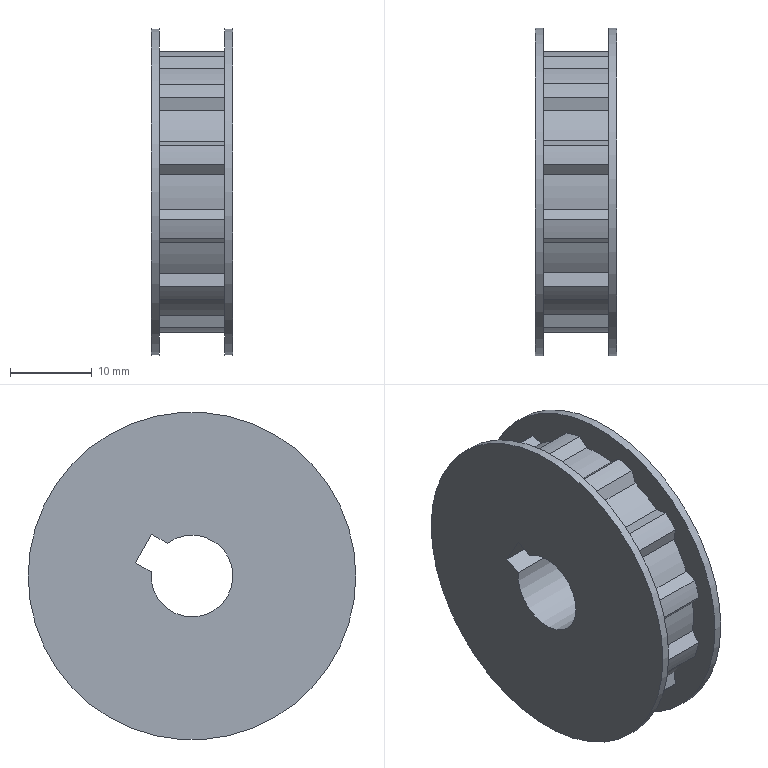Part | NX | features DATUM_CSYS 4, EXTRUDE 3, SKETCH 3, Container 1, EXTRACT_BODY 1, Geometry Instance 1, UNITE 1 | 1 solid | 58 faces | box 10 x 40 x 40 mm | volume 8689 mm3 | plane 31 | cylinder 27 | commonest cylinder face diameters 32.525 x12 35 x12 40 x2 10 x1